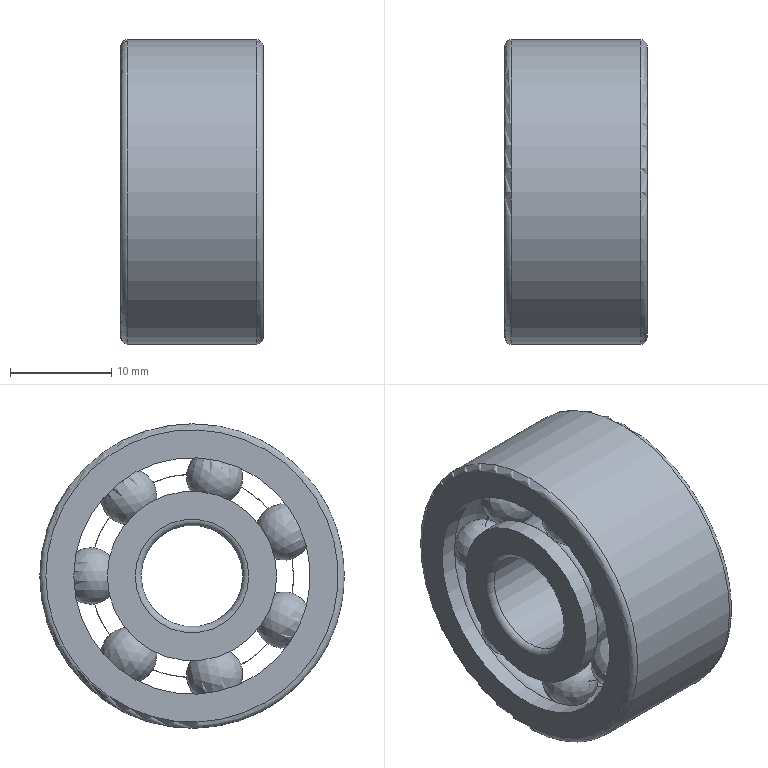Part | NX | features skf_bearing_4200_atn9_2_1 5 | 4 solids | 48 faces | box 14 x 30 x 30 mm | volume 6245 mm3 | torus 22 | sphere 14 | cylinder 8 | plane 4 | commonest cylinder face diameters 16.7 x3 23.3 x3 10 x1 30 x1